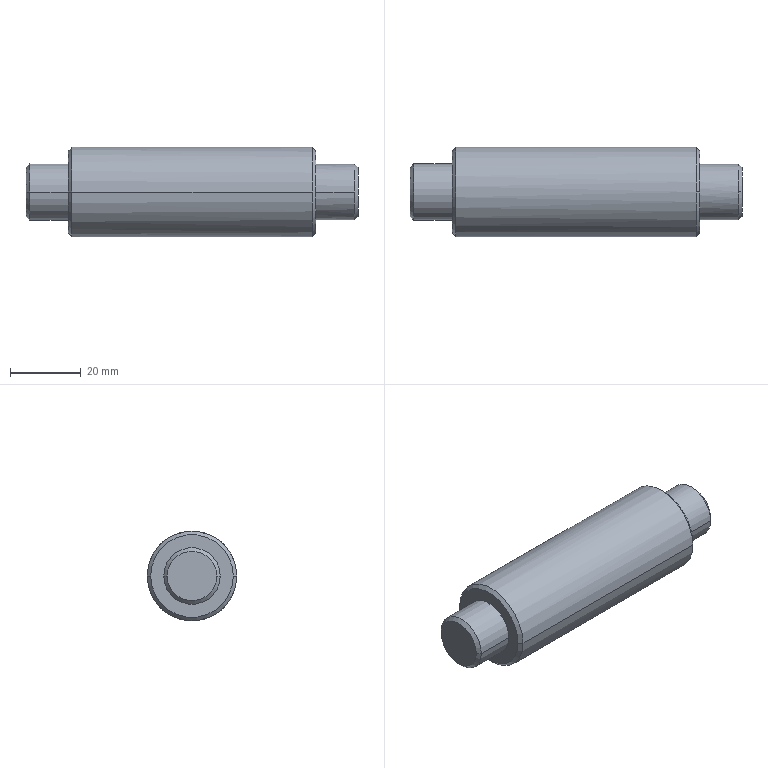Part | SolidWorks | features BaseBody 1 | 1 solid | 18 faces | box 94 x 25.4 x 25.4 mm | volume 40077 mm3 | cone 8 | cylinder 6 | plane 4 | commonest cylinder face diameters 15.691 x2 16 x2 25.4 x2
STEP:
#1=CARTESIAN_POINT('',(2.709,12.506,0.));
#2=VERTEX_POINT('',#1);
#3=CARTESIAN_POINT('',(2.709,-12.894,0.));
#4=VERTEX_POINT('',#3);
#5=CARTESIAN_POINT('',(2.709,-0.1942,0.));
#6=DIRECTION('',(1.,0.,0.));
#7=DIRECTION('',(0.,1.,0.));
#8=AXIS2_PLACEMENT_3D('',#5,#6,#7);
#9=CIRCLE('',#8,12.7);
#10=EDGE_CURVE('',#2,#4,#9,.T.);
#11=ORIENTED_EDGE('',*,*,#10,.T.);
#12=CARTESIAN_POINT('',(70.709,-12.894,0.));
#13=VERTEX_POINT('',#12);
#14=CARTESIAN_POINT('',(36.709,-12.894,0.));
#15=DIRECTION('',(1.,0.,0.));
#16=VECTOR('',#15,1000.);
#17=LINE('',#14,#16);
#18=EDGE_CURVE('',#4,#13,#17,.T.);
#19=ORIENTED_EDGE('',*,*,#18,.T.);
#20=CARTESIAN_POINT('',(70.709,-0.1942,12.7));
#21=VERTEX_POINT('',#20);
#22=CARTESIAN_POINT('',(70.709,-0.1942,0.));
#23=DIRECTION('',(-1.,0.,0.));
#24=DIRECTION('',(0.,1.,0.));
#25=AXIS2_PLACEMENT_3D('',#22,#23,#24);
#26=CIRCLE('',#25,12.7);
#27=EDGE_CURVE('',#13,#21,#26,.T.);
#28=ORIENTED_EDGE('',*,*,#27,.T.);
#29=CARTESIAN_POINT('',(70.709,12.506,0.));
#30=VERTEX_POINT('',#29);
#31=CARTESIAN_POINT('',(70.709,-0.1942,0.));
#32=DIRECTION('',(-1.,0.,0.));
#33=DIRECTION('',(0.,1.,0.));
#34=AXIS2_PLACEMENT_3D('',#31,#32,#33);
#35=CIRCLE('',#34,12.7);
#36=EDGE_CURVE('',#21,#30,#35,.T.);
#37=ORIENTED_EDGE('',*,*,#36,.T.);
#38=CARTESIAN_POINT('',(36.709,12.506,0.));
#39=DIRECTION('',(1.,0.,0.));
#40=VECTOR('',#39,1000.);
#41=LINE('',#38,#40);
#42=EDGE_CURVE('',#2,#30,#41,.T.);
#43=ORIENTED_EDGE('',*,*,#42,.F.);
#44=EDGE_LOOP('',(#11,#19,#28,#37,#43));
#45=FACE_OUTER_BOUND('',#44,.T.);
#46=CARTESIAN_POINT('',(36.709,-0.1942,0.));
#47=DIRECTION('',(1.,0.,0.));
#48=DIRECTION('',(0.,1.,0.));
#49=AXIS2_PLACEMENT_3D('',#46,#47,#48);
#50=CYLINDRICAL_SURFACE('',#49,12.7);
#51=ADVANCED_FACE('',(#45),#50,.T.);
#52=CARTESIAN_POINT('',(71.709,-0.1942,11.7));
#53=VERTEX_POINT('',#52);
#54=CARTESIAN_POINT('',(71.709,-0.1942,-11.7));
#55=VERTEX_POINT('',#54);
#56=CARTESIAN_POINT('',(71.709,-0.1942,0.));
#57=DIRECTION('',(-1.,0.,0.));
#58=DIRECTION('',(0.,0.,1.));
#59=AXIS2_PLACEMENT_3D('',#56,#57,#58);
#60=CIRCLE('',#59,11.7);
#61=EDGE_CURVE('',#53,#55,#60,.T.);
#62=ORIENTED_EDGE('',*,*,#61,.T.);
#63=CARTESIAN_POINT('',(70.709,-0.1942,-12.7));
#64=VERTEX_POINT('',#63);
#65=CARTESIAN_POINT('',(70.709,-0.1942,-12.7));
#66=DIRECTION('',(-0.7071,0.,-0.7071));
#67=VECTOR('',#66,1000.);
#68=LINE('',#65,#67);
#69=EDGE_CURVE('',#55,#64,#68,.T.);
#70=ORIENTED_EDGE('',*,*,#69,.T.);
#71=CARTESIAN_POINT('',(70.709,-0.1942,0.));
#72=DIRECTION('',(-1.,0.,0.));
#73=DIRECTION('',(0.,1.,0.));
#74=AXIS2_PLACEMENT_3D('',#71,#72,#73);
#75=CIRCLE('',#74,12.7);
#76=EDGE_CURVE('',#30,#64,#75,.T.);
#77=ORIENTED_EDGE('',*,*,#76,.F.);
#78=ORIENTED_EDGE('',*,*,#36,.F.);
#79=CARTESIAN_POINT('',(70.709,-0.1942,12.7));
#80=DIRECTION('',(-0.7071,0.,0.7071));
#81=VECTOR('',#80,1000.);
#82=LINE('',#79,#81);
#83=EDGE_CURVE('',#53,#21,#82,.T.);
#84=ORIENTED_EDGE('',*,*,#83,.F.);
#85=EDGE_LOOP('',(#62,#70,#77,#78,#84));
#86=FACE_OUTER_BOUND('',#85,.T.);
#87=CARTESIAN_POINT('',(70.709,-0.1942,0.));
#88=DIRECTION('',(-1.,0.,0.));
#89=DIRECTION('',(0.,0.,1.));
#90=AXIS2_PLACEMENT_3D('',#87,#88,#89);
#91=CONICAL_SURFACE('',#90,12.7,0.7854);
#92=ADVANCED_FACE('',(#86),#91,.T.);
#93=CARTESIAN_POINT('',(1.709,11.506,0.));
#94=VERTEX_POINT('',#93);
#95=CARTESIAN_POINT('',(1.709,-11.894,0.));
#96=VERTEX_POINT('',#95);
#97=CARTESIAN_POINT('',(1.709,-0.1942,0.));
#98=DIRECTION('',(1.,0.,0.));
#99=DIRECTION('',(0.,1.,0.));
#100=AXIS2_PLACEMENT_3D('',#97,#98,#99);
#101=CIRCLE('',#100,11.7);
#102=EDGE_CURVE('',#94,#96,#101,.T.);
#103=ORIENTED_EDGE('',*,*,#102,.T.);
#104=CARTESIAN_POINT('',(2.709,-12.894,0.));
#105=DIRECTION('',(0.7071,-0.7071,0.));
#106=VECTOR('',#105,1000.);
#107=LINE('',#104,#106);
#108=EDGE_CURVE('',#96,#4,#107,.T.);
#109=ORIENTED_EDGE('',*,*,#108,.T.);
#110=ORIENTED_EDGE('',*,*,#10,.F.);
#111=CARTESIAN_POINT('',(2.709,12.506,0.));
#112=DIRECTION('',(0.7071,0.7071,0.));
#113=VECTOR('',#112,1000.);
#114=LINE('',#111,#113);
#115=EDGE_CURVE('',#94,#2,#114,.T.);
#116=ORIENTED_EDGE('',*,*,#115,.F.);
#117=EDGE_LOOP('',(#103,#109,#110,#116));
#118=FACE_OUTER_BOUND('',#117,.T.);
#119=CARTESIAN_POINT('',(2.709,-0.1942,0.));
#120=DIRECTION('',(1.,0.,0.));
#121=DIRECTION('',(0.,1.,0.));
#122=AXIS2_PLACEMENT_3D('',#119,#120,#121);
#123=CONICAL_SURFACE('',#122,12.7,0.7854);
#124=ADVANCED_FACE('',(#118),#123,.T.);
#125=CARTESIAN_POINT('',(71.709,-8.04,0.));
#126=VERTEX_POINT('',#125);
#127=CARTESIAN_POINT('',(71.709,7.651,0.));
#128=VERTEX_POINT('',#127);
#129=CARTESIAN_POINT('',(71.709,-0.1942,0.));
#130=DIRECTION('',(-1.,0.,0.));
#131=DIRECTION('',(0.,1.,0.));
#132=AXIS2_PLACEMENT_3D('',#129,#130,#131);
#133=CIRCLE('',#132,7.846);
#134=EDGE_CURVE('',#126,#128,#133,.T.);
#135=ORIENTED_EDGE('',*,*,#134,.F.);
#136=CARTESIAN_POINT('',(82.709,-8.04,0.));
#137=VERTEX_POINT('',#136);
#138=CARTESIAN_POINT('',(77.709,-8.04,0.));
#139=DIRECTION('',(1.,0.,0.));
#140=VECTOR('',#139,1000.);
#141=LINE('',#138,#140);
#142=EDGE_CURVE('',#126,#137,#141,.T.);
#143=ORIENTED_EDGE('',*,*,#142,.T.);
#144=CARTESIAN_POINT('',(82.709,-0.1942,7.846));
#145=VERTEX_POINT('',#144);
#146=CARTESIAN_POINT('',(82.709,-0.1942,0.));
#147=DIRECTION('',(-1.,0.,0.));
#148=DIRECTION('',(0.,1.,0.));
#149=AXIS2_PLACEMENT_3D('',#146,#147,#148);
#150=CIRCLE('',#149,7.846);
#151=EDGE_CURVE('',#137,#145,#150,.T.);
#152=ORIENTED_EDGE('',*,*,#151,.T.);
#153=CARTESIAN_POINT('',(82.709,7.651,0.));
#154=VERTEX_POINT('',#153);
#155=CARTESIAN_POINT('',(82.709,-0.1942,0.));
#156=DIRECTION('',(-1.,0.,0.));
#157=DIRECTION('',(0.,1.,0.));
#158=AXIS2_PLACEMENT_3D('',#155,#156,#157);
#159=CIRCLE('',#158,7.846);
#160=EDGE_CURVE('',#145,#154,#159,.T.);
#161=ORIENTED_EDGE('',*,*,#160,.T.);
#162=CARTESIAN_POINT('',(77.709,7.651,0.));
#163=DIRECTION('',(1.,0.,0.));
#164=VECTOR('',#163,1000.);
#165=LINE('',#162,#164);
#166=EDGE_CURVE('',#128,#154,#165,.T.);
#167=ORIENTED_EDGE('',*,*,#166,.F.);
#168=EDGE_LOOP('',(#135,#143,#152,#161,#167));
#169=FACE_OUTER_BOUND('',#168,.T.);
#170=CARTESIAN_POINT('',(77.709,-0.1942,0.));
#171=DIRECTION('',(1.,0.,0.));
#172=DIRECTION('',(0.,1.,0.));
#173=AXIS2_PLACEMENT_3D('',#170,#171,#172);
#174=CYLINDRICAL_SURFACE('',#173,7.846);
#175=ADVANCED_FACE('',(#169),#174,.T.);
#176=CARTESIAN_POINT('',(-9.291,7.806,0.));
#177=VERTEX_POINT('',#176);
#178=CARTESIAN_POINT('',(-9.291,-8.194,0.));
#179=VERTEX_POINT('',#178);
#180=CARTESIAN_POINT('',(-9.291,-0.1942,0.));
#181=DIRECTION('',(1.,0.,0.));
#182=DIRECTION('',(0.,1.,0.));
#183=AXIS2_PLACEMENT_3D('',#180,#181,#182);
#184=CIRCLE('',#183,8.);
#185=EDGE_CURVE('',#177,#179,#184,.T.);
#186=ORIENTED_EDGE('',*,*,#185,.T.);
#187=CARTESIAN_POINT('',(1.709,-8.194,0.));
#188=VERTEX_POINT('',#187);
#189=CARTESIAN_POINT('',(-4.291,-8.194,0.));
#190=DIRECTION('',(1.,0.,0.));
#191=VECTOR('',#190,1000.);
#192=LINE('',#189,#191);
#193=EDGE_CURVE('',#179,#188,#192,.T.);
#194=ORIENTED_EDGE('',*,*,#193,.T.);
#195=CARTESIAN_POINT('',(1.709,7.806,0.));
#196=VERTEX_POINT('',#195);
#197=CARTESIAN_POINT('',(1.709,-0.1942,0.));
#198=DIRECTION('',(1.,0.,0.));
#199=DIRECTION('',(0.,1.,0.));
#200=AXIS2_PLACEMENT_3D('',#197,#198,#199);
#201=CIRCLE('',#200,8.);
#202=EDGE_CURVE('',#196,#188,#201,.T.);
#203=ORIENTED_EDGE('',*,*,#202,.F.);
#204=CARTESIAN_POINT('',(-4.291,7.806,0.));
#205=DIRECTION('',(1.,0.,0.));
#206=VECTOR('',#205,1000.);
#207=LINE('',#204,#206);
#208=EDGE_CURVE('',#177,#196,#207,.T.);
#209=ORIENTED_EDGE('',*,*,#208,.F.);
#210=EDGE_LOOP('',(#186,#194,#203,#209));
#211=FACE_OUTER_BOUND('',#210,.T.);
#212=CARTESIAN_POINT('',(-4.291,-0.1942,0.));
#213=DIRECTION('',(1.,0.,0.));
#214=DIRECTION('',(0.,1.,0.));
#215=AXIS2_PLACEMENT_3D('',#212,#213,#214);
#216=CYLINDRICAL_SURFACE('',#215,8.);
#217=ADVANCED_FACE('',(#211),#216,.T.);
#218=CARTESIAN_POINT('',(83.709,-0.1942,6.846));
#219=VERTEX_POINT('',#218);
#220=CARTESIAN_POINT('',(83.709,-0.1942,-6.846));
#221=VERTEX_POINT('',#220);
#222=CARTESIAN_POINT('',(83.709,-0.1942,0.));
#223=DIRECTION('',(-1.,0.,0.));
#224=DIRECTION('',(0.,0.,1.));
#225=AXIS2_PLACEMENT_3D('',#222,#223,#224);
#226=CIRCLE('',#225,6.846);
#227=EDGE_CURVE('',#219,#221,#226,.T.);
#228=ORIENTED_EDGE('',*,*,#227,.T.);
#229=CARTESIAN_POINT('',(82.709,-0.1942,-7.846));
#230=VERTEX_POINT('',#229);
#231=CARTESIAN_POINT('',(82.709,-0.1942,-7.846));
#232=DIRECTION('',(-0.7071,0.,-0.7071));
#233=VECTOR('',#232,1000.);
#234=LINE('',#231,#233);
#235=EDGE_CURVE('',#221,#230,#234,.T.);
#236=ORIENTED_EDGE('',*,*,#235,.T.);
#237=CARTESIAN_POINT('',(82.709,-0.1942,0.));
#238=DIRECTION('',(-1.,0.,0.));
#239=DIRECTION('',(0.,1.,0.));
#240=AXIS2_PLACEMENT_3D('',#237,#238,#239);
#241=CIRCLE('',#240,7.846);
#242=EDGE_CURVE('',#154,#230,#241,.T.);
#243=ORIENTED_EDGE('',*,*,#242,.F.);
#244=ORIENTED_EDGE('',*,*,#160,.F.);
#245=CARTESIAN_POINT('',(82.709,-0.1942,7.846));
#246=DIRECTION('',(-0.7071,0.,0.7071));
#247=VECTOR('',#246,1000.);
#248=LINE('',#245,#247);
#249=EDGE_CURVE('',#219,#145,#248,.T.);
#250=ORIENTED_EDGE('',*,*,#249,.F.);
#251=EDGE_LOOP('',(#228,#236,#243,#244,#250));
#252=FACE_OUTER_BOUND('',#251,.T.);
#253=CARTESIAN_POINT('',(82.709,-0.1942,0.));
#254=DIRECTION('',(-1.,0.,0.));
#255=DIRECTION('',(0.,0.,1.));
#256=AXIS2_PLACEMENT_3D('',#253,#254,#255);
#257=CONICAL_SURFACE('',#256,7.846,0.7854);
#258=ADVANCED_FACE('',(#252),#257,.T.);
#259=CARTESIAN_POINT('',(-10.291,6.806,0.));
#260=VERTEX_POINT('',#259);
#261=CARTESIAN_POINT('',(-10.291,-7.194,0.));
#262=VERTEX_POINT('',#261);
#263=CARTESIAN_POINT('',(-10.291,-0.1942,0.));
#264=DIRECTION('',(1.,0.,0.));
#265=DIRECTION('',(0.,1.,0.));
#266=AXIS2_PLACEMENT_3D('',#263,#264,#265);
#267=CIRCLE('',#266,7.);
#268=EDGE_CURVE('',#260,#262,#267,.T.);
#269=ORIENTED_EDGE('',*,*,#268,.T.);
#270=CARTESIAN_POINT('',(-9.291,-8.194,0.));
#271=DIRECTION('',(0.7071,-0.7071,0.));
#272=VECTOR('',#271,1000.);
#273=LINE('',#270,#272);
#274=EDGE_CURVE('',#262,#179,#273,.T.);
#275=ORIENTED_EDGE('',*,*,#274,.T.);
#276=ORIENTED_EDGE('',*,*,#185,.F.);
#277=CARTESIAN_POINT('',(-9.291,7.806,0.));
#278=DIRECTION('',(0.7071,0.7071,0.));
#279=VECTOR('',#278,1000.);
#280=LINE('',#277,#279);
#281=EDGE_CURVE('',#260,#177,#280,.T.);
#282=ORIENTED_EDGE('',*,*,#281,.F.);
#283=EDGE_LOOP('',(#269,#275,#276,#282));
#284=FACE_OUTER_BOUND('',#283,.T.);
#285=CARTESIAN_POINT('',(-9.291,-0.1942,0.));
#286=DIRECTION('',(1.,0.,0.));
#287=DIRECTION('',(0.,1.,0.));
#288=AXIS2_PLACEMENT_3D('',#285,#286,#287);
#289=CONICAL_SURFACE('',#288,8.,0.7854);
#290=ADVANCED_FACE('',(#284),#289,.T.);
#291=ORIENTED_EDGE('',*,*,#18,.F.);
#292=CARTESIAN_POINT('',(2.709,-0.1942,0.));
#293=DIRECTION('',(1.,0.,0.));
#294=DIRECTION('',(0.,1.,0.));
#295=AXIS2_PLACEMENT_3D('',#292,#293,#294);
#296=CIRCLE('',#295,12.7);
#297=EDGE_CURVE('',#4,#2,#296,.T.);
#298=ORIENTED_EDGE('',*,*,#297,.T.);
#299=ORIENTED_EDGE('',*,*,#42,.T.);
#300=ORIENTED_EDGE('',*,*,#76,.T.);
#301=CARTESIAN_POINT('',(70.709,-0.1942,0.));
#302=DIRECTION('',(-1.,0.,0.));
#303=DIRECTION('',(0.,1.,0.));
#304=AXIS2_PLACEMENT_3D('',#301,#302,#303);
#305=CIRCLE('',#304,12.7);
#306=EDGE_CURVE('',#64,#13,#305,.T.);
#307=ORIENTED_EDGE('',*,*,#306,.T.);
#308=EDGE_LOOP('',(#291,#298,#299,#300,#307));
#309=FACE_OUTER_BOUND('',#308,.T.);
#310=CARTESIAN_POINT('',(36.709,-0.1942,0.));
#311=DIRECTION('',(1.,0.,0.));
#312=DIRECTION('',(0.,1.,0.));
#313=AXIS2_PLACEMENT_3D('',#310,#311,#312);
#314=CYLINDRICAL_SURFACE('',#313,12.7);
#315=ADVANCED_FACE('',(#309),#314,.T.);
#316=ORIENTED_EDGE('',*,*,#69,.F.);
#317=CARTESIAN_POINT('',(71.709,-0.1942,0.));
#318=DIRECTION('',(-1.,0.,0.));
#319=DIRECTION('',(0.,0.,1.));
#320=AXIS2_PLACEMENT_3D('',#317,#318,#319);
#321=CIRCLE('',#320,11.7);
#322=EDGE_CURVE('',#55,#53,#321,.T.);
#323=ORIENTED_EDGE('',*,*,#322,.T.);
#324=ORIENTED_EDGE('',*,*,#83,.T.);
#325=ORIENTED_EDGE('',*,*,#27,.F.);
#326=ORIENTED_EDGE('',*,*,#306,.F.);
#327=EDGE_LOOP('',(#316,#323,#324,#325,#326));
#328=FACE_OUTER_BOUND('',#327,.T.);
#329=CARTESIAN_POINT('',(70.709,-0.1942,0.));
#330=DIRECTION('',(-1.,0.,0.));
#331=DIRECTION('',(0.,0.,1.));
#332=AXIS2_PLACEMENT_3D('',#329,#330,#331);
#333=CONICAL_SURFACE('',#332,12.7,0.7854);
#334=ADVANCED_FACE('',(#328),#333,.T.);
#335=ORIENTED_EDGE('',*,*,#108,.F.);
#336=CARTESIAN_POINT('',(1.709,-0.1942,0.));
#337=DIRECTION('',(1.,0.,0.));
#338=DIRECTION('',(0.,1.,0.));
#339=AXIS2_PLACEMENT_3D('',#336,#337,#338);
#340=CIRCLE('',#339,11.7);
#341=EDGE_CURVE('',#96,#94,#340,.T.);
#342=ORIENTED_EDGE('',*,*,#341,.T.);
#343=ORIENTED_EDGE('',*,*,#115,.T.);
#344=ORIENTED_EDGE('',*,*,#297,.F.);
#345=EDGE_LOOP('',(#335,#342,#343,#344));
#346=FACE_OUTER_BOUND('',#345,.T.);
#347=CARTESIAN_POINT('',(2.709,-0.1942,0.));
#348=DIRECTION('',(1.,0.,0.));
#349=DIRECTION('',(0.,1.,0.));
#350=AXIS2_PLACEMENT_3D('',#347,#348,#349);
#351=CONICAL_SURFACE('',#350,12.7,0.7854);
#352=ADVANCED_FACE('',(#346),#351,.T.);
#353=CARTESIAN_POINT('',(71.709,-0.1942,0.));
#354=DIRECTION('',(-1.,0.,0.));
#355=DIRECTION('',(0.,1.,0.));
#356=AXIS2_PLACEMENT_3D('',#353,#354,#355);
#357=CIRCLE('',#356,7.846);
#358=EDGE_CURVE('',#128,#126,#357,.T.);
#359=ORIENTED_EDGE('',*,*,#358,.T.);
#360=ORIENTED_EDGE('',*,*,#134,.T.);
#361=EDGE_LOOP('',(#359,#360));
#362=FACE_BOUND('',#361,.T.);
#363=ORIENTED_EDGE('',*,*,#61,.F.);
#364=ORIENTED_EDGE('',*,*,#322,.F.);
#365=EDGE_LOOP('',(#363,#364));
#366=FACE_OUTER_BOUND('',#365,.T.);
#367=CARTESIAN_POINT('',(71.709,10.079,0.));
#368=DIRECTION('',(1.,0.,0.));
#369=DIRECTION('',(0.,1.,0.));
#370=AXIS2_PLACEMENT_3D('',#367,#368,#369);
#371=PLANE('',#370);
#372=ADVANCED_FACE('',(#362,#366),#371,.T.);
#373=ORIENTED_EDGE('',*,*,#202,.T.);
#374=CARTESIAN_POINT('',(1.709,-0.1942,0.));
#375=DIRECTION('',(1.,0.,0.));
#376=DIRECTION('',(0.,1.,0.));
#377=AXIS2_PLACEMENT_3D('',#374,#375,#376);
#378=CIRCLE('',#377,8.);
#379=EDGE_CURVE('',#188,#196,#378,.T.);
#380=ORIENTED_EDGE('',*,*,#379,.T.);
#381=EDGE_LOOP('',(#373,#380));
#382=FACE_BOUND('',#381,.T.);
#383=ORIENTED_EDGE('',*,*,#102,.F.);
#384=ORIENTED_EDGE('',*,*,#341,.F.);
#385=EDGE_LOOP('',(#383,#384));
#386=FACE_OUTER_BOUND('',#385,.T.);
#387=CARTESIAN_POINT('',(1.709,10.156,0.));
#388=DIRECTION('',(-1.,0.,0.));
#389=DIRECTION('',(0.,-1.,0.));
#390=AXIS2_PLACEMENT_3D('',#387,#388,#389);
#391=PLANE('',#390);
#392=ADVANCED_FACE('',(#382,#386),#391,.T.);
#393=ORIENTED_EDGE('',*,*,#142,.F.);
#394=ORIENTED_EDGE('',*,*,#358,.F.);
#395=ORIENTED_EDGE('',*,*,#166,.T.);
#396=ORIENTED_EDGE('',*,*,#242,.T.);
#397=CARTESIAN_POINT('',(82.709,-0.1942,0.));
#398=DIRECTION('',(-1.,0.,0.));
#399=DIRECTION('',(0.,1.,0.));
#400=AXIS2_PLACEMENT_3D('',#397,#398,#399);
#401=CIRCLE('',#400,7.846);
#402=EDGE_CURVE('',#230,#137,#401,.T.);
#403=ORIENTED_EDGE('',*,*,#402,.T.);
#404=EDGE_LOOP('',(#393,#394,#395,#396,#403));
#405=FACE_OUTER_BOUND('',#404,.T.);
#406=CARTESIAN_POINT('',(77.709,-0.1942,0.));
#407=DIRECTION('',(1.,0.,0.));
#408=DIRECTION('',(0.,1.,0.));
#409=AXIS2_PLACEMENT_3D('',#406,#407,#408);
#410=CYLINDRICAL_SURFACE('',#409,7.846);
#411=ADVANCED_FACE('',(#405),#410,.T.);
#412=ORIENTED_EDGE('',*,*,#193,.F.);
#413=CARTESIAN_POINT('',(-9.291,-0.1942,0.));
#414=DIRECTION('',(1.,0.,0.));
#415=DIRECTION('',(0.,1.,0.));
#416=AXIS2_PLACEMENT_3D('',#413,#414,#415);
#417=CIRCLE('',#416,8.);
#418=EDGE_CURVE('',#179,#177,#417,.T.);
#419=ORIENTED_EDGE('',*,*,#418,.T.);
#420=ORIENTED_EDGE('',*,*,#208,.T.);
#421=ORIENTED_EDGE('',*,*,#379,.F.);
#422=EDGE_LOOP('',(#412,#419,#420,#421));
#423=FACE_OUTER_BOUND('',#422,.T.);
#424=CARTESIAN_POINT('',(-4.291,-0.1942,0.));
#425=DIRECTION('',(1.,0.,0.));
#426=DIRECTION('',(0.,1.,0.));
#427=AXIS2_PLACEMENT_3D('',#424,#425,#426);
#428=CYLINDRICAL_SURFACE('',#427,8.);
#429=ADVANCED_FACE('',(#423),#428,.T.);
#430=ORIENTED_EDGE('',*,*,#235,.F.);
#431=CARTESIAN_POINT('',(83.709,-0.1942,0.));
#432=DIRECTION('',(-1.,0.,0.));
#433=DIRECTION('',(0.,0.,1.));
#434=AXIS2_PLACEMENT_3D('',#431,#432,#433);
#435=CIRCLE('',#434,6.846);
#436=EDGE_CURVE('',#221,#219,#435,.T.);
#437=ORIENTED_EDGE('',*,*,#436,.T.);
#438=ORIENTED_EDGE('',*,*,#249,.T.);
#439=ORIENTED_EDGE('',*,*,#151,.F.);
#440=ORIENTED_EDGE('',*,*,#402,.F.);
#441=EDGE_LOOP('',(#430,#437,#438,#439,#440));
#442=FACE_OUTER_BOUND('',#441,.T.);
#443=CARTESIAN_POINT('',(82.709,-0.1942,0.));
#444=DIRECTION('',(-1.,0.,0.));
#445=DIRECTION('',(0.,0.,1.));
#446=AXIS2_PLACEMENT_3D('',#443,#444,#445);
#447=CONICAL_SURFACE('',#446,7.846,0.7854);
#448=ADVANCED_FACE('',(#442),#447,.T.);
#449=ORIENTED_EDGE('',*,*,#274,.F.);
#450=CARTESIAN_POINT('',(-10.291,-0.1942,0.));
#451=DIRECTION('',(1.,0.,0.));
#452=DIRECTION('',(0.,1.,0.));
#453=AXIS2_PLACEMENT_3D('',#450,#451,#452);
#454=CIRCLE('',#453,7.);
#455=EDGE_CURVE('',#262,#260,#454,.T.);
#456=ORIENTED_EDGE('',*,*,#455,.T.);
#457=ORIENTED_EDGE('',*,*,#281,.T.);
#458=ORIENTED_EDGE('',*,*,#418,.F.);
#459=EDGE_LOOP('',(#449,#456,#457,#458));
#460=FACE_OUTER_BOUND('',#459,.T.);
#461=CARTESIAN_POINT('',(-9.291,-0.1942,0.));
#462=DIRECTION('',(1.,0.,0.));
#463=DIRECTION('',(0.,1.,0.));
#464=AXIS2_PLACEMENT_3D('',#461,#462,#463);
#465=CONICAL_SURFACE('',#464,8.,0.7854);
#466=ADVANCED_FACE('',(#460),#465,.T.);
#467=ORIENTED_EDGE('',*,*,#227,.F.);
#468=ORIENTED_EDGE('',*,*,#436,.F.);
#469=EDGE_LOOP('',(#467,#468));
#470=FACE_OUTER_BOUND('',#469,.T.);
#471=CARTESIAN_POINT('',(83.709,3.729,0.));
#472=DIRECTION('',(1.,0.,0.));
#473=DIRECTION('',(0.,1.,0.));
#474=AXIS2_PLACEMENT_3D('',#471,#472,#473);
#475=PLANE('',#474);
#476=ADVANCED_FACE('',(#470),#475,.T.);
#477=ORIENTED_EDGE('',*,*,#268,.F.);
#478=ORIENTED_EDGE('',*,*,#455,.F.);
#479=EDGE_LOOP('',(#477,#478));
#480=FACE_OUTER_BOUND('',#479,.T.);
#481=CARTESIAN_POINT('',(-10.291,3.806,0.));
#482=DIRECTION('',(-1.,0.,0.));
#483=DIRECTION('',(0.,-1.,0.));
#484=AXIS2_PLACEMENT_3D('',#481,#482,#483);
#485=PLANE('',#484);
#486=ADVANCED_FACE('',(#480),#485,.T.);
#487=CLOSED_SHELL('',(#51,#92,#124,#175,#217,#258,#290,#315,#334,#352,#372,#392,#411,#429,#448,#466,#476,#486));
#488=MANIFOLD_SOLID_BREP('',#487);
#489=CARTESIAN_POINT('',(0.,0.,0.));
#490=DIRECTION('',(0.,0.,1.));
#491=DIRECTION('',(1.,0.,0.));
#492=AXIS2_PLACEMENT_3D('',#489,#490,#491);
#493=(LENGTH_UNIT()NAMED_UNIT(*)SI_UNIT(.MILLI.,.METRE.));
#494=UNCERTAINTY_MEASURE_WITH_UNIT(LENGTH_MEASURE(0.00001),#493,'','');
#495=(NAMED_UNIT(*)PLANE_ANGLE_UNIT()SI_UNIT($,.RADIAN.));
#496=(NAMED_UNIT(*)SI_UNIT($,.STERADIAN.)SOLID_ANGLE_UNIT());
#497=(GEOMETRIC_REPRESENTATION_CONTEXT(3)GLOBAL_UNCERTAINTY_ASSIGNED_CONTEXT((#494))GLOBAL_UNIT_ASSIGNED_CONTEXT((#493,#495,#496))REPRESENTATION_CONTEXT('',''));
#498=ADVANCED_BREP_SHAPE_REPRESENTATION('',(#488,#492),#497);